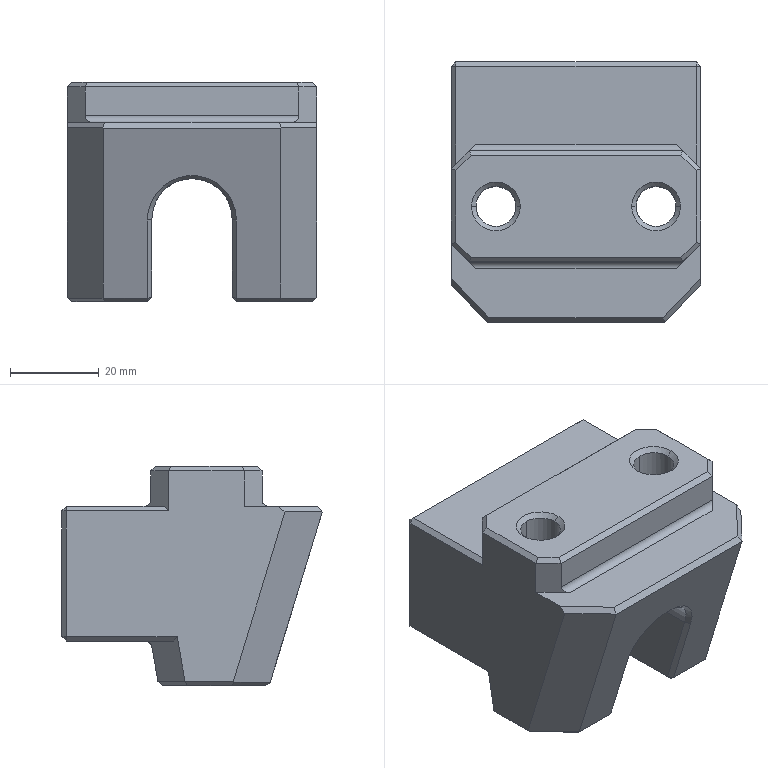Part | Creo | 1 solid | 98 faces | box 56 x 58.503 x 49.267 mm | volume 88566 mm3 | plane 73 | cylinder 13 | cone 11 | spline 1 | commonest cylinder face diameters 3 x4 9 x4 14 x4 18 x1